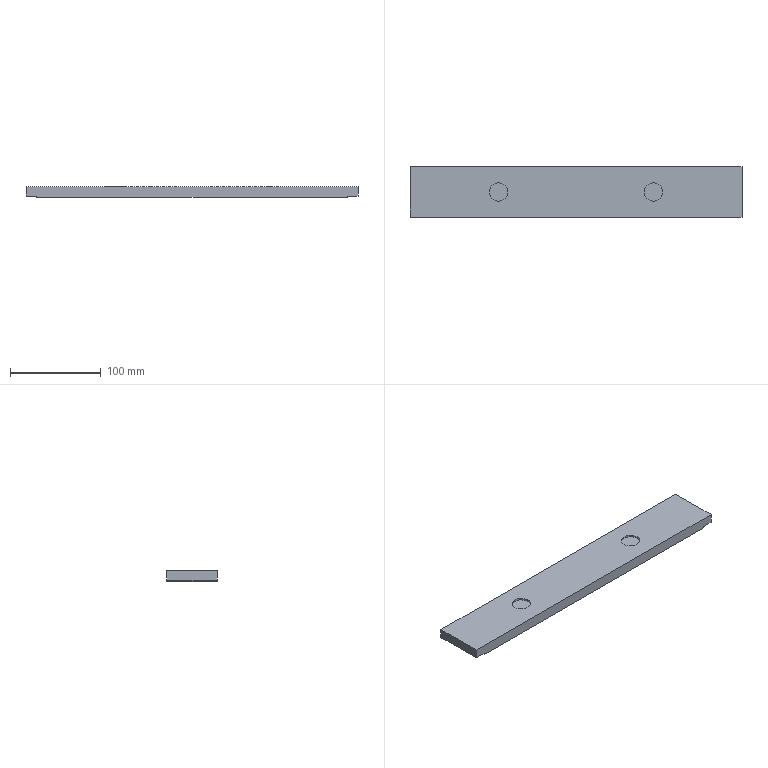Part | SolidWorks | features ICE 2, Extrusion 1 | 1 solid | 16 faces | box 365 x 55 x 12 mm | volume 237663 mm3 | plane 12 | cylinder 4 | commonest cylinder face diameters 20 x4
STEP:
#1=CARTESIAN_POINT('',(75.,0.,10.));
#2=VERTEX_POINT('',#1);
#3=CARTESIAN_POINT('',(95.,0.,10.));
#4=VERTEX_POINT('',#3);
#5=CARTESIAN_POINT('',(85.,0.,10.));
#6=DIRECTION('',(0.,0.,1.));
#7=DIRECTION('',(1.,0.,0.));
#8=AXIS2_PLACEMENT_3D('',#5,#6,#7);
#9=CIRCLE('',#8,10.);
#10=EDGE_CURVE('',#2,#4,#9,.T.);
#11=ORIENTED_EDGE('',*,*,#10,.F.);
#12=CARTESIAN_POINT('',(75.,0.,12.));
#13=VERTEX_POINT('',#12);
#14=CARTESIAN_POINT('',(75.,0.,10.));
#15=DIRECTION('',(0.,0.,1.));
#16=VECTOR('',#15,1000.);
#17=LINE('',#14,#16);
#18=EDGE_CURVE('',#2,#13,#17,.T.);
#19=ORIENTED_EDGE('',*,*,#18,.T.);
#20=CARTESIAN_POINT('',(95.,0.,12.));
#21=VERTEX_POINT('',#20);
#22=CARTESIAN_POINT('',(85.,0.,12.));
#23=DIRECTION('',(0.,0.,1.));
#24=DIRECTION('',(1.,0.,0.));
#25=AXIS2_PLACEMENT_3D('',#22,#23,#24);
#26=CIRCLE('',#25,10.);
#27=EDGE_CURVE('',#13,#21,#26,.T.);
#28=ORIENTED_EDGE('',*,*,#27,.T.);
#29=CARTESIAN_POINT('',(95.,0.,10.));
#30=DIRECTION('',(0.,0.,1.));
#31=VECTOR('',#30,1000.);
#32=LINE('',#29,#31);
#33=EDGE_CURVE('',#4,#21,#32,.T.);
#34=ORIENTED_EDGE('',*,*,#33,.F.);
#35=EDGE_LOOP('',(#11,#19,#28,#34));
#36=FACE_OUTER_BOUND('',#35,.T.);
#37=CARTESIAN_POINT('',(85.,0.,10.));
#38=DIRECTION('',(0.,0.,1.));
#39=DIRECTION('',(1.,0.,0.));
#40=AXIS2_PLACEMENT_3D('',#37,#38,#39);
#41=CYLINDRICAL_SURFACE('',#40,10.);
#42=ADVANCED_FACE('',(#36),#41,.F.);
#43=CARTESIAN_POINT('',(-95.,0.,10.));
#44=VERTEX_POINT('',#43);
#45=CARTESIAN_POINT('',(-75.,0.,10.));
#46=VERTEX_POINT('',#45);
#47=CARTESIAN_POINT('',(-85.,0.,10.));
#48=DIRECTION('',(0.,0.,1.));
#49=DIRECTION('',(1.,0.,0.));
#50=AXIS2_PLACEMENT_3D('',#47,#48,#49);
#51=CIRCLE('',#50,10.);
#52=EDGE_CURVE('',#44,#46,#51,.T.);
#53=ORIENTED_EDGE('',*,*,#52,.F.);
#54=CARTESIAN_POINT('',(-95.,0.,12.));
#55=VERTEX_POINT('',#54);
#56=CARTESIAN_POINT('',(-95.,0.,10.));
#57=DIRECTION('',(0.,0.,1.));
#58=VECTOR('',#57,1000.);
#59=LINE('',#56,#58);
#60=EDGE_CURVE('',#44,#55,#59,.T.);
#61=ORIENTED_EDGE('',*,*,#60,.T.);
#62=CARTESIAN_POINT('',(-75.,0.,12.));
#63=VERTEX_POINT('',#62);
#64=CARTESIAN_POINT('',(-85.,0.,12.));
#65=DIRECTION('',(0.,0.,1.));
#66=DIRECTION('',(1.,0.,0.));
#67=AXIS2_PLACEMENT_3D('',#64,#65,#66);
#68=CIRCLE('',#67,10.);
#69=EDGE_CURVE('',#55,#63,#68,.T.);
#70=ORIENTED_EDGE('',*,*,#69,.T.);
#71=CARTESIAN_POINT('',(-75.,0.,10.));
#72=DIRECTION('',(0.,0.,1.));
#73=VECTOR('',#72,1000.);
#74=LINE('',#71,#73);
#75=EDGE_CURVE('',#46,#63,#74,.T.);
#76=ORIENTED_EDGE('',*,*,#75,.F.);
#77=EDGE_LOOP('',(#53,#61,#70,#76));
#78=FACE_OUTER_BOUND('',#77,.T.);
#79=CARTESIAN_POINT('',(-85.,0.,10.));
#80=DIRECTION('',(0.,0.,1.));
#81=DIRECTION('',(1.,0.,0.));
#82=AXIS2_PLACEMENT_3D('',#79,#80,#81);
#83=CYLINDRICAL_SURFACE('',#82,10.);
#84=ADVANCED_FACE('',(#78),#83,.F.);
#85=CARTESIAN_POINT('',(-182.5,-27.5,1.5));
#86=VERTEX_POINT('',#85);
#87=CARTESIAN_POINT('',(-182.5,27.5,1.5));
#88=VERTEX_POINT('',#87);
#89=CARTESIAN_POINT('',(-182.5,-27.5,1.5));
#90=DIRECTION('',(0.,1.,0.));
#91=VECTOR('',#90,1000.);
#92=LINE('',#89,#91);
#93=EDGE_CURVE('',#86,#88,#92,.T.);
#94=ORIENTED_EDGE('',*,*,#93,.F.);
#95=CARTESIAN_POINT('',(-182.5,-27.5,12.));
#96=VERTEX_POINT('',#95);
#97=CARTESIAN_POINT('',(-182.5,-27.5,12.));
#98=DIRECTION('',(0.,0.,-1.));
#99=VECTOR('',#98,1000.);
#100=LINE('',#97,#99);
#101=EDGE_CURVE('',#96,#86,#100,.T.);
#102=ORIENTED_EDGE('',*,*,#101,.F.);
#103=CARTESIAN_POINT('',(-182.5,27.5,12.));
#104=VERTEX_POINT('',#103);
#105=CARTESIAN_POINT('',(-182.5,-27.5,12.));
#106=DIRECTION('',(0.,-1.,0.));
#107=VECTOR('',#106,1000.);
#108=LINE('',#105,#107);
#109=EDGE_CURVE('',#104,#96,#108,.T.);
#110=ORIENTED_EDGE('',*,*,#109,.F.);
#111=CARTESIAN_POINT('',(-182.5,27.5,12.));
#112=DIRECTION('',(0.,0.,-1.));
#113=VECTOR('',#112,1000.);
#114=LINE('',#111,#113);
#115=EDGE_CURVE('',#104,#88,#114,.T.);
#116=ORIENTED_EDGE('',*,*,#115,.T.);
#117=EDGE_LOOP('',(#94,#102,#110,#116));
#118=FACE_OUTER_BOUND('',#117,.T.);
#119=CARTESIAN_POINT('',(-182.5,-27.5,12.));
#120=DIRECTION('',(1.,0.,0.));
#121=DIRECTION('',(0.,0.,-1.));
#122=AXIS2_PLACEMENT_3D('',#119,#120,#121);
#123=PLANE('',#122);
#124=ADVANCED_FACE('',(#118),#123,.F.);
#125=CARTESIAN_POINT('',(182.5,-27.5,12.));
#126=VERTEX_POINT('',#125);
#127=CARTESIAN_POINT('',(182.5,-27.5,1.5));
#128=VERTEX_POINT('',#127);
#129=CARTESIAN_POINT('',(182.5,-27.5,12.));
#130=DIRECTION('',(0.,0.,-1.));
#131=VECTOR('',#130,1000.);
#132=LINE('',#129,#131);
#133=EDGE_CURVE('',#126,#128,#132,.T.);
#134=ORIENTED_EDGE('',*,*,#133,.T.);
#135=CARTESIAN_POINT('',(182.5,27.5,1.5));
#136=VERTEX_POINT('',#135);
#137=CARTESIAN_POINT('',(182.5,-27.5,1.5));
#138=DIRECTION('',(0.,-1.,0.));
#139=VECTOR('',#138,1000.);
#140=LINE('',#137,#139);
#141=EDGE_CURVE('',#136,#128,#140,.T.);
#142=ORIENTED_EDGE('',*,*,#141,.F.);
#143=CARTESIAN_POINT('',(182.5,27.5,12.));
#144=VERTEX_POINT('',#143);
#145=CARTESIAN_POINT('',(182.5,27.5,12.));
#146=DIRECTION('',(0.,0.,-1.));
#147=VECTOR('',#146,1000.);
#148=LINE('',#145,#147);
#149=EDGE_CURVE('',#144,#136,#148,.T.);
#150=ORIENTED_EDGE('',*,*,#149,.F.);
#151=CARTESIAN_POINT('',(182.5,-27.5,12.));
#152=DIRECTION('',(0.,1.,0.));
#153=VECTOR('',#152,1000.);
#154=LINE('',#151,#153);
#155=EDGE_CURVE('',#126,#144,#154,.T.);
#156=ORIENTED_EDGE('',*,*,#155,.F.);
#157=EDGE_LOOP('',(#134,#142,#150,#156));
#158=FACE_OUTER_BOUND('',#157,.T.);
#159=CARTESIAN_POINT('',(182.5,-27.5,12.));
#160=DIRECTION('',(-1.,0.,0.));
#161=DIRECTION('',(0.,0.,1.));
#162=AXIS2_PLACEMENT_3D('',#159,#160,#161);
#163=PLANE('',#162);
#164=ADVANCED_FACE('',(#158),#163,.F.);
#165=CARTESIAN_POINT('',(170.5,27.5,0.));
#166=VERTEX_POINT('',#165);
#167=CARTESIAN_POINT('',(-170.5,27.5,0.));
#168=VERTEX_POINT('',#167);
#169=CARTESIAN_POINT('',(-182.5,27.5,0.));
#170=DIRECTION('',(-1.,0.,0.));
#171=VECTOR('',#170,1000.);
#172=LINE('',#169,#171);
#173=EDGE_CURVE('',#166,#168,#172,.T.);
#174=ORIENTED_EDGE('',*,*,#173,.T.);
#175=CARTESIAN_POINT('',(-170.5,27.5,1.5));
#176=VERTEX_POINT('',#175);
#177=CARTESIAN_POINT('',(-170.5,27.5,1.5));
#178=DIRECTION('',(0.,0.,-1.));
#179=VECTOR('',#178,1000.);
#180=LINE('',#177,#179);
#181=EDGE_CURVE('',#176,#168,#180,.T.);
#182=ORIENTED_EDGE('',*,*,#181,.F.);
#183=CARTESIAN_POINT('',(-182.5,27.5,1.5));
#184=DIRECTION('',(1.,0.,0.));
#185=VECTOR('',#184,1000.);
#186=LINE('',#183,#185);
#187=EDGE_CURVE('',#88,#176,#186,.T.);
#188=ORIENTED_EDGE('',*,*,#187,.F.);
#189=ORIENTED_EDGE('',*,*,#115,.F.);
#190=CARTESIAN_POINT('',(-182.5,27.5,12.));
#191=DIRECTION('',(-1.,0.,0.));
#192=VECTOR('',#191,1000.);
#193=LINE('',#190,#192);
#194=EDGE_CURVE('',#144,#104,#193,.T.);
#195=ORIENTED_EDGE('',*,*,#194,.F.);
#196=ORIENTED_EDGE('',*,*,#149,.T.);
#197=CARTESIAN_POINT('',(170.5,27.5,1.5));
#198=VERTEX_POINT('',#197);
#199=CARTESIAN_POINT('',(182.5,27.5,1.5));
#200=DIRECTION('',(1.,0.,0.));
#201=VECTOR('',#200,1000.);
#202=LINE('',#199,#201);
#203=EDGE_CURVE('',#198,#136,#202,.T.);
#204=ORIENTED_EDGE('',*,*,#203,.F.);
#205=CARTESIAN_POINT('',(170.5,27.5,1.5));
#206=DIRECTION('',(0.,0.,-1.));
#207=VECTOR('',#206,1000.);
#208=LINE('',#205,#207);
#209=EDGE_CURVE('',#198,#166,#208,.T.);
#210=ORIENTED_EDGE('',*,*,#209,.T.);
#211=EDGE_LOOP('',(#174,#182,#188,#189,#195,#196,#204,#210));
#212=FACE_OUTER_BOUND('',#211,.T.);
#213=CARTESIAN_POINT('',(-182.5,27.5,12.));
#214=DIRECTION('',(0.,-1.,0.));
#215=DIRECTION('',(0.,0.,-1.));
#216=AXIS2_PLACEMENT_3D('',#213,#214,#215);
#217=PLANE('',#216);
#218=ADVANCED_FACE('',(#212),#217,.F.);
#219=CARTESIAN_POINT('',(-170.5,-27.5,1.5));
#220=VERTEX_POINT('',#219);
#221=CARTESIAN_POINT('',(-182.5,-27.5,1.5));
#222=DIRECTION('',(-1.,0.,0.));
#223=VECTOR('',#222,1000.);
#224=LINE('',#221,#223);
#225=EDGE_CURVE('',#220,#86,#224,.T.);
#226=ORIENTED_EDGE('',*,*,#225,.F.);
#227=CARTESIAN_POINT('',(-170.5,-27.5,0.));
#228=VERTEX_POINT('',#227);
#229=CARTESIAN_POINT('',(-170.5,-27.5,1.5));
#230=DIRECTION('',(0.,0.,-1.));
#231=VECTOR('',#230,1000.);
#232=LINE('',#229,#231);
#233=EDGE_CURVE('',#220,#228,#232,.T.);
#234=ORIENTED_EDGE('',*,*,#233,.T.);
#235=CARTESIAN_POINT('',(170.5,-27.5,0.));
#236=VERTEX_POINT('',#235);
#237=CARTESIAN_POINT('',(-182.5,-27.5,0.));
#238=DIRECTION('',(1.,0.,0.));
#239=VECTOR('',#238,1000.);
#240=LINE('',#237,#239);
#241=EDGE_CURVE('',#228,#236,#240,.T.);
#242=ORIENTED_EDGE('',*,*,#241,.T.);
#243=CARTESIAN_POINT('',(170.5,-27.5,1.5));
#244=VERTEX_POINT('',#243);
#245=CARTESIAN_POINT('',(170.5,-27.5,1.5));
#246=DIRECTION('',(0.,0.,-1.));
#247=VECTOR('',#246,1000.);
#248=LINE('',#245,#247);
#249=EDGE_CURVE('',#244,#236,#248,.T.);
#250=ORIENTED_EDGE('',*,*,#249,.F.);
#251=CARTESIAN_POINT('',(182.5,-27.5,1.5));
#252=DIRECTION('',(-1.,0.,0.));
#253=VECTOR('',#252,1000.);
#254=LINE('',#251,#253);
#255=EDGE_CURVE('',#128,#244,#254,.T.);
#256=ORIENTED_EDGE('',*,*,#255,.F.);
#257=ORIENTED_EDGE('',*,*,#133,.F.);
#258=CARTESIAN_POINT('',(-182.5,-27.5,12.));
#259=DIRECTION('',(1.,0.,0.));
#260=VECTOR('',#259,1000.);
#261=LINE('',#258,#260);
#262=EDGE_CURVE('',#96,#126,#261,.T.);
#263=ORIENTED_EDGE('',*,*,#262,.F.);
#264=ORIENTED_EDGE('',*,*,#101,.T.);
#265=EDGE_LOOP('',(#226,#234,#242,#250,#256,#257,#263,#264));
#266=FACE_OUTER_BOUND('',#265,.T.);
#267=CARTESIAN_POINT('',(-182.5,-27.5,12.));
#268=DIRECTION('',(0.,1.,0.));
#269=DIRECTION('',(0.,0.,1.));
#270=AXIS2_PLACEMENT_3D('',#267,#268,#269);
#271=PLANE('',#270);
#272=ADVANCED_FACE('',(#266),#271,.F.);
#273=CARTESIAN_POINT('',(85.,0.,12.));
#274=DIRECTION('',(0.,0.,1.));
#275=DIRECTION('',(1.,0.,0.));
#276=AXIS2_PLACEMENT_3D('',#273,#274,#275);
#277=CIRCLE('',#276,10.);
#278=EDGE_CURVE('',#21,#13,#277,.T.);
#279=ORIENTED_EDGE('',*,*,#278,.F.);
#280=ORIENTED_EDGE('',*,*,#27,.F.);
#281=EDGE_LOOP('',(#279,#280));
#282=FACE_BOUND('',#281,.T.);
#283=CARTESIAN_POINT('',(-85.,0.,12.));
#284=DIRECTION('',(0.,0.,1.));
#285=DIRECTION('',(1.,0.,0.));
#286=AXIS2_PLACEMENT_3D('',#283,#284,#285);
#287=CIRCLE('',#286,10.);
#288=EDGE_CURVE('',#63,#55,#287,.T.);
#289=ORIENTED_EDGE('',*,*,#288,.F.);
#290=ORIENTED_EDGE('',*,*,#69,.F.);
#291=EDGE_LOOP('',(#289,#290));
#292=FACE_BOUND('',#291,.T.);
#293=ORIENTED_EDGE('',*,*,#155,.T.);
#294=ORIENTED_EDGE('',*,*,#194,.T.);
#295=ORIENTED_EDGE('',*,*,#109,.T.);
#296=ORIENTED_EDGE('',*,*,#262,.T.);
#297=EDGE_LOOP('',(#293,#294,#295,#296));
#298=FACE_OUTER_BOUND('',#297,.T.);
#299=CARTESIAN_POINT('',(0.,0.,12.));
#300=DIRECTION('',(0.,0.,-1.));
#301=DIRECTION('',(-1.,0.,0.));
#302=AXIS2_PLACEMENT_3D('',#299,#300,#301);
#303=PLANE('',#302);
#304=ADVANCED_FACE('',(#282,#292,#298),#303,.F.);
#305=CARTESIAN_POINT('',(-170.5,-27.5,0.));
#306=DIRECTION('',(0.,-1.,0.));
#307=VECTOR('',#306,1000.);
#308=LINE('',#305,#307);
#309=EDGE_CURVE('',#168,#228,#308,.T.);
#310=ORIENTED_EDGE('',*,*,#309,.F.);
#311=ORIENTED_EDGE('',*,*,#173,.F.);
#312=CARTESIAN_POINT('',(170.5,-27.5,0.));
#313=DIRECTION('',(0.,1.,0.));
#314=VECTOR('',#313,1000.);
#315=LINE('',#312,#314);
#316=EDGE_CURVE('',#236,#166,#315,.T.);
#317=ORIENTED_EDGE('',*,*,#316,.F.);
#318=ORIENTED_EDGE('',*,*,#241,.F.);
#319=EDGE_LOOP('',(#310,#311,#317,#318));
#320=FACE_OUTER_BOUND('',#319,.T.);
#321=CARTESIAN_POINT('',(0.,0.,0.));
#322=DIRECTION('',(0.,0.,-1.));
#323=DIRECTION('',(-1.,0.,0.));
#324=AXIS2_PLACEMENT_3D('',#321,#322,#323);
#325=PLANE('',#324);
#326=ADVANCED_FACE('',(#320),#325,.T.);
#327=ORIENTED_EDGE('',*,*,#60,.F.);
#328=CARTESIAN_POINT('',(-85.,0.,10.));
#329=DIRECTION('',(0.,0.,1.));
#330=DIRECTION('',(1.,0.,0.));
#331=AXIS2_PLACEMENT_3D('',#328,#329,#330);
#332=CIRCLE('',#331,10.);
#333=EDGE_CURVE('',#46,#44,#332,.T.);
#334=ORIENTED_EDGE('',*,*,#333,.F.);
#335=ORIENTED_EDGE('',*,*,#75,.T.);
#336=ORIENTED_EDGE('',*,*,#288,.T.);
#337=EDGE_LOOP('',(#327,#334,#335,#336));
#338=FACE_OUTER_BOUND('',#337,.T.);
#339=CARTESIAN_POINT('',(-85.,0.,10.));
#340=DIRECTION('',(0.,0.,1.));
#341=DIRECTION('',(1.,0.,0.));
#342=AXIS2_PLACEMENT_3D('',#339,#340,#341);
#343=CYLINDRICAL_SURFACE('',#342,10.);
#344=ADVANCED_FACE('',(#338),#343,.F.);
#345=ORIENTED_EDGE('',*,*,#333,.T.);
#346=ORIENTED_EDGE('',*,*,#52,.T.);
#347=EDGE_LOOP('',(#345,#346));
#348=FACE_OUTER_BOUND('',#347,.T.);
#349=CARTESIAN_POINT('',(-85.,0.,10.));
#350=DIRECTION('',(0.,0.,1.));
#351=DIRECTION('',(1.,0.,0.));
#352=AXIS2_PLACEMENT_3D('',#349,#350,#351);
#353=PLANE('',#352);
#354=ADVANCED_FACE('',(#348),#353,.T.);
#355=ORIENTED_EDGE('',*,*,#18,.F.);
#356=CARTESIAN_POINT('',(85.,0.,10.));
#357=DIRECTION('',(0.,0.,1.));
#358=DIRECTION('',(1.,0.,0.));
#359=AXIS2_PLACEMENT_3D('',#356,#357,#358);
#360=CIRCLE('',#359,10.);
#361=EDGE_CURVE('',#4,#2,#360,.T.);
#362=ORIENTED_EDGE('',*,*,#361,.F.);
#363=ORIENTED_EDGE('',*,*,#33,.T.);
#364=ORIENTED_EDGE('',*,*,#278,.T.);
#365=EDGE_LOOP('',(#355,#362,#363,#364));
#366=FACE_OUTER_BOUND('',#365,.T.);
#367=CARTESIAN_POINT('',(85.,0.,10.));
#368=DIRECTION('',(0.,0.,1.));
#369=DIRECTION('',(1.,0.,0.));
#370=AXIS2_PLACEMENT_3D('',#367,#368,#369);
#371=CYLINDRICAL_SURFACE('',#370,10.);
#372=ADVANCED_FACE('',(#366),#371,.F.);
#373=ORIENTED_EDGE('',*,*,#361,.T.);
#374=ORIENTED_EDGE('',*,*,#10,.T.);
#375=EDGE_LOOP('',(#373,#374));
#376=FACE_OUTER_BOUND('',#375,.T.);
#377=CARTESIAN_POINT('',(85.,0.,10.));
#378=DIRECTION('',(0.,0.,1.));
#379=DIRECTION('',(1.,0.,0.));
#380=AXIS2_PLACEMENT_3D('',#377,#378,#379);
#381=PLANE('',#380);
#382=ADVANCED_FACE('',(#376),#381,.T.);
#383=ORIENTED_EDGE('',*,*,#316,.T.);
#384=ORIENTED_EDGE('',*,*,#209,.F.);
#385=CARTESIAN_POINT('',(170.5,-27.5,1.5));
#386=DIRECTION('',(0.,1.,0.));
#387=VECTOR('',#386,1000.);
#388=LINE('',#385,#387);
#389=EDGE_CURVE('',#244,#198,#388,.T.);
#390=ORIENTED_EDGE('',*,*,#389,.F.);
#391=ORIENTED_EDGE('',*,*,#249,.T.);
#392=EDGE_LOOP('',(#383,#384,#390,#391));
#393=FACE_OUTER_BOUND('',#392,.T.);
#394=CARTESIAN_POINT('',(170.5,-27.5,1.5));
#395=DIRECTION('',(-1.,0.,0.));
#396=DIRECTION('',(0.,0.,1.));
#397=AXIS2_PLACEMENT_3D('',#394,#395,#396);
#398=PLANE('',#397);
#399=ADVANCED_FACE('',(#393),#398,.F.);
#400=ORIENTED_EDGE('',*,*,#141,.T.);
#401=ORIENTED_EDGE('',*,*,#255,.T.);
#402=ORIENTED_EDGE('',*,*,#389,.T.);
#403=ORIENTED_EDGE('',*,*,#203,.T.);
#404=EDGE_LOOP('',(#400,#401,#402,#403));
#405=FACE_OUTER_BOUND('',#404,.T.);
#406=CARTESIAN_POINT('',(0.,0.,1.5));
#407=DIRECTION('',(0.,0.,1.));
#408=DIRECTION('',(1.,0.,0.));
#409=AXIS2_PLACEMENT_3D('',#406,#407,#408);
#410=PLANE('',#409);
#411=ADVANCED_FACE('',(#405),#410,.F.);
#412=ORIENTED_EDGE('',*,*,#309,.T.);
#413=ORIENTED_EDGE('',*,*,#233,.F.);
#414=CARTESIAN_POINT('',(-170.5,-27.5,1.5));
#415=DIRECTION('',(0.,-1.,0.));
#416=VECTOR('',#415,1000.);
#417=LINE('',#414,#416);
#418=EDGE_CURVE('',#176,#220,#417,.T.);
#419=ORIENTED_EDGE('',*,*,#418,.F.);
#420=ORIENTED_EDGE('',*,*,#181,.T.);
#421=EDGE_LOOP('',(#412,#413,#419,#420));
#422=FACE_OUTER_BOUND('',#421,.T.);
#423=CARTESIAN_POINT('',(-170.5,-27.5,1.5));
#424=DIRECTION('',(1.,0.,0.));
#425=DIRECTION('',(0.,0.,-1.));
#426=AXIS2_PLACEMENT_3D('',#423,#424,#425);
#427=PLANE('',#426);
#428=ADVANCED_FACE('',(#422),#427,.F.);
#429=ORIENTED_EDGE('',*,*,#93,.T.);
#430=ORIENTED_EDGE('',*,*,#187,.T.);
#431=ORIENTED_EDGE('',*,*,#418,.T.);
#432=ORIENTED_EDGE('',*,*,#225,.T.);
#433=EDGE_LOOP('',(#429,#430,#431,#432));
#434=FACE_OUTER_BOUND('',#433,.T.);
#435=CARTESIAN_POINT('',(0.,0.,1.5));
#436=DIRECTION('',(0.,0.,-1.));
#437=DIRECTION('',(-1.,0.,0.));
#438=AXIS2_PLACEMENT_3D('',#435,#436,#437);
#439=PLANE('',#438);
#440=ADVANCED_FACE('',(#434),#439,.T.);
#441=CLOSED_SHELL('',(#42,#84,#124,#164,#218,#272,#304,#326,#344,#354,#372,#382,#399,#411,#428,#440));
#442=MANIFOLD_SOLID_BREP('',#441);
#443=CARTESIAN_POINT('',(0.,0.,0.));
#444=DIRECTION('',(0.,0.,1.));
#445=DIRECTION('',(1.,0.,0.));
#446=AXIS2_PLACEMENT_3D('',#443,#444,#445);
#447=(LENGTH_UNIT()NAMED_UNIT(*)SI_UNIT(.MILLI.,.METRE.));
#448=UNCERTAINTY_MEASURE_WITH_UNIT(LENGTH_MEASURE(0.00001),#447,'','');
#449=(NAMED_UNIT(*)PLANE_ANGLE_UNIT()SI_UNIT($,.RADIAN.));
#450=(NAMED_UNIT(*)SI_UNIT($,.STERADIAN.)SOLID_ANGLE_UNIT());
#451=(GEOMETRIC_REPRESENTATION_CONTEXT(3)GLOBAL_UNCERTAINTY_ASSIGNED_CONTEXT((#448))GLOBAL_UNIT_ASSIGNED_CONTEXT((#447,#449,#450))REPRESENTATION_CONTEXT('',''));
#452=ADVANCED_BREP_SHAPE_REPRESENTATION('',(#442,#446),#451);